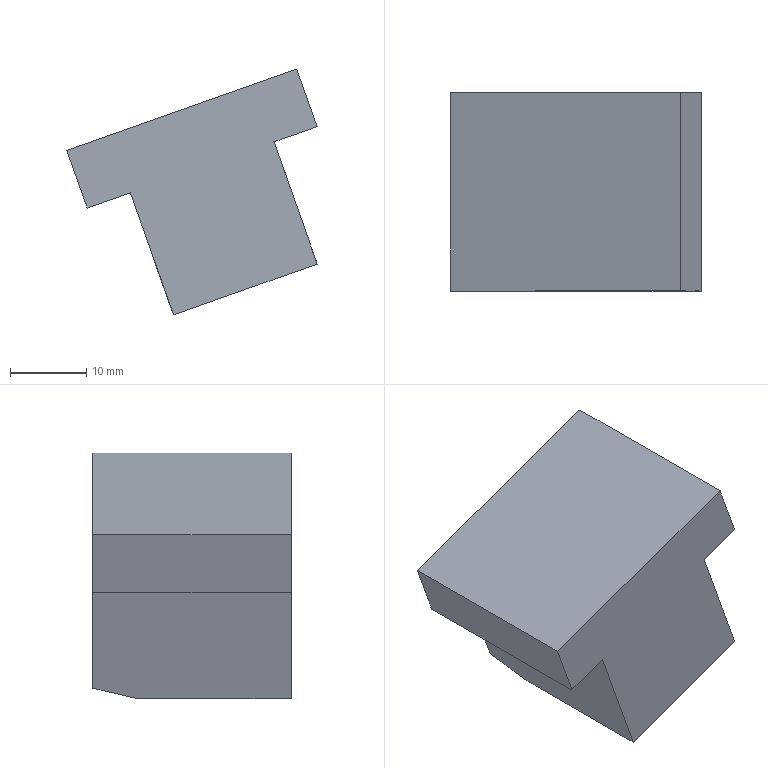Part | STEP file | T-BLOCK1_id174_x_t | 1 solid | 11 faces | box 32.854 x 26 x 32.245 mm | volume 15406 mm3 | plane 11
STEP:
#1=CARTESIAN_POINT('',(48.232,-40.,-222.441));
#2=VERTEX_POINT('',#1);
#3=CARTESIAN_POINT('',(67.085,-40.,-215.765));
#4=VERTEX_POINT('',#3);
#5=CARTESIAN_POINT('',(67.085,-40.,-215.765));
#6=DIRECTION('',(0.9426,0.,0.3338));
#7=VECTOR('',#6,1.);
#8=LINE('',#5,#7);
#9=EDGE_CURVE('',#2,#4,#8,.T.);
#10=ORIENTED_EDGE('',*,*,#9,.F.);
#11=CARTESIAN_POINT('',(47.733,-34.,-221.031));
#12=VERTEX_POINT('',#11);
#13=CARTESIAN_POINT('',(47.733,-34.,-221.031));
#14=DIRECTION('',(0.08076,-0.9703,-0.228));
#15=VECTOR('',#14,1.);
#16=LINE('',#13,#15);
#17=EDGE_CURVE('',#12,#2,#16,.T.);
#18=ORIENTED_EDGE('',*,*,#17,.F.);
#19=CARTESIAN_POINT('',(66.586,-34.,-214.355));
#20=VERTEX_POINT('',#19);
#21=CARTESIAN_POINT('',(66.586,-34.,-214.355));
#22=DIRECTION('',(-0.9426,0.,-0.3338));
#23=VECTOR('',#22,1.);
#24=LINE('',#21,#23);
#25=EDGE_CURVE('',#20,#12,#24,.T.);
#26=ORIENTED_EDGE('',*,*,#25,.F.);
#27=CARTESIAN_POINT('',(67.085,-40.,-215.765));
#28=DIRECTION('',(-0.08076,0.9703,0.228));
#29=VECTOR('',#28,1.);
#30=LINE('',#27,#29);
#31=EDGE_CURVE('',#4,#20,#30,.T.);
#32=ORIENTED_EDGE('',*,*,#31,.F.);
#33=EDGE_LOOP('',(#10,#18,#26,#32));
#34=FACE_OUTER_BOUND('',#33,.T.);
#35=CARTESIAN_POINT('',(1.1,-40.,-239.131));
#36=DIRECTION('',(-0.3239,-0.2419,0.9146));
#37=DIRECTION('',(0.9426,0.,0.3338));
#38=AXIS2_PLACEMENT_3D('',#35,#36,#37);
#39=PLANE('',#38);
#40=ADVANCED_FACE('',(#34),#39,.F.);
#41=CARTESIAN_POINT('',(48.232,-60.,-222.441));
#42=VERTEX_POINT('',#41);
#43=CARTESIAN_POINT('',(48.232,-60.,-222.441));
#44=DIRECTION('',(0.,-1.,0.));
#45=VECTOR('',#44,1.);
#46=LINE('',#43,#45);
#47=EDGE_CURVE('',#2,#42,#46,.T.);
#48=ORIENTED_EDGE('',*,*,#47,.F.);
#49=ORIENTED_EDGE('',*,*,#9,.T.);
#50=CARTESIAN_POINT('',(67.085,-60.,-215.765));
#51=VERTEX_POINT('',#50);
#52=CARTESIAN_POINT('',(67.085,-60.,-215.765));
#53=DIRECTION('',(0.,1.,0.));
#54=VECTOR('',#53,1.);
#55=LINE('',#52,#54);
#56=EDGE_CURVE('',#51,#4,#55,.T.);
#57=ORIENTED_EDGE('',*,*,#56,.F.);
#58=CARTESIAN_POINT('',(67.085,-60.,-215.765));
#59=DIRECTION('',(-0.9426,0.,-0.3338));
#60=VECTOR('',#59,1.);
#61=LINE('',#58,#60);
#62=EDGE_CURVE('',#51,#42,#61,.T.);
#63=ORIENTED_EDGE('',*,*,#62,.T.);
#64=EDGE_LOOP('',(#48,#49,#57,#63));
#65=FACE_OUTER_BOUND('',#64,.T.);
#66=CARTESIAN_POINT('',(67.085,-60.,-215.765));
#67=DIRECTION('',(0.3338,0.,-0.9426));
#68=DIRECTION('',(-0.9426,0.,-0.3338));
#69=AXIS2_PLACEMENT_3D('',#66,#67,#68);
#70=PLANE('',#69);
#71=ADVANCED_FACE('',(#65),#70,.T.);
#72=CARTESIAN_POINT('',(42.558,-34.,-206.416));
#73=VERTEX_POINT('',#72);
#74=CARTESIAN_POINT('',(47.733,-34.,-221.031));
#75=DIRECTION('',(-0.3338,0.,0.9426));
#76=VECTOR('',#75,1.);
#77=LINE('',#74,#76);
#78=EDGE_CURVE('',#12,#73,#77,.T.);
#79=ORIENTED_EDGE('',*,*,#78,.F.);
#80=ORIENTED_EDGE('',*,*,#17,.T.);
#81=ORIENTED_EDGE('',*,*,#47,.T.);
#82=CARTESIAN_POINT('',(42.558,-60.,-206.416));
#83=VERTEX_POINT('',#82);
#84=CARTESIAN_POINT('',(48.232,-60.,-222.441));
#85=DIRECTION('',(-0.3338,0.,0.9426));
#86=VECTOR('',#85,1.);
#87=LINE('',#84,#86);
#88=EDGE_CURVE('',#42,#83,#87,.T.);
#89=ORIENTED_EDGE('',*,*,#88,.T.);
#90=CARTESIAN_POINT('',(42.558,-60.,-206.416));
#91=DIRECTION('',(0.,-1.,0.));
#92=VECTOR('',#91,1.);
#93=LINE('',#90,#92);
#94=EDGE_CURVE('',#73,#83,#93,.T.);
#95=ORIENTED_EDGE('',*,*,#94,.F.);
#96=EDGE_LOOP('',(#79,#80,#81,#89,#95));
#97=FACE_OUTER_BOUND('',#96,.T.);
#98=CARTESIAN_POINT('',(48.232,-60.,-222.441));
#99=DIRECTION('',(-0.9426,0.,-0.3338));
#100=DIRECTION('',(-0.3338,0.,0.9426));
#101=AXIS2_PLACEMENT_3D('',#98,#99,#100);
#102=PLANE('',#101);
#103=ADVANCED_FACE('',(#97),#102,.T.);
#104=ORIENTED_EDGE('',*,*,#94,.T.);
#105=CARTESIAN_POINT('',(36.902,-60.,-208.419));
#106=VERTEX_POINT('',#105);
#107=CARTESIAN_POINT('',(42.558,-60.,-206.416));
#108=DIRECTION('',(-0.9426,0.,-0.3338));
#109=VECTOR('',#108,1.);
#110=LINE('',#107,#109);
#111=EDGE_CURVE('',#83,#106,#110,.T.);
#112=ORIENTED_EDGE('',*,*,#111,.T.);
#113=CARTESIAN_POINT('',(36.902,-34.,-208.419));
#114=VERTEX_POINT('',#113);
#115=CARTESIAN_POINT('',(36.902,-60.,-208.419));
#116=DIRECTION('',(0.,-1.,0.));
#117=VECTOR('',#116,1.);
#118=LINE('',#115,#117);
#119=EDGE_CURVE('',#114,#106,#118,.T.);
#120=ORIENTED_EDGE('',*,*,#119,.F.);
#121=CARTESIAN_POINT('',(42.558,-34.,-206.416));
#122=DIRECTION('',(-0.9426,0.,-0.3338));
#123=VECTOR('',#122,1.);
#124=LINE('',#121,#123);
#125=EDGE_CURVE('',#73,#114,#124,.T.);
#126=ORIENTED_EDGE('',*,*,#125,.F.);
#127=EDGE_LOOP('',(#104,#112,#120,#126));
#128=FACE_OUTER_BOUND('',#127,.T.);
#129=CARTESIAN_POINT('',(42.558,-60.,-206.416));
#130=DIRECTION('',(0.3338,0.,-0.9426));
#131=DIRECTION('',(-0.9426,0.,-0.3338));
#132=AXIS2_PLACEMENT_3D('',#129,#130,#131);
#133=PLANE('',#132);
#134=ADVANCED_FACE('',(#128),#133,.T.);
#135=CARTESIAN_POINT('',(67.066,-60.,-197.737));
#136=VERTEX_POINT('',#135);
#137=CARTESIAN_POINT('',(67.066,-34.,-197.737));
#138=VERTEX_POINT('',#137);
#139=CARTESIAN_POINT('',(67.066,-60.,-197.737));
#140=DIRECTION('',(0.,1.,0.));
#141=VECTOR('',#140,1.);
#142=LINE('',#139,#141);
#143=EDGE_CURVE('',#136,#138,#142,.T.);
#144=ORIENTED_EDGE('',*,*,#143,.F.);
#145=CARTESIAN_POINT('',(61.41,-60.,-199.74));
#146=VERTEX_POINT('',#145);
#147=CARTESIAN_POINT('',(67.066,-60.,-197.737));
#148=DIRECTION('',(-0.9426,0.,-0.3338));
#149=VECTOR('',#148,1.);
#150=LINE('',#147,#149);
#151=EDGE_CURVE('',#136,#146,#150,.T.);
#152=ORIENTED_EDGE('',*,*,#151,.T.);
#153=CARTESIAN_POINT('',(61.41,-34.,-199.74));
#154=VERTEX_POINT('',#153);
#155=CARTESIAN_POINT('',(61.41,-60.,-199.74));
#156=DIRECTION('',(0.,-1.,0.));
#157=VECTOR('',#156,1.);
#158=LINE('',#155,#157);
#159=EDGE_CURVE('',#154,#146,#158,.T.);
#160=ORIENTED_EDGE('',*,*,#159,.F.);
#161=CARTESIAN_POINT('',(67.066,-34.,-197.737));
#162=DIRECTION('',(-0.9426,0.,-0.3338));
#163=VECTOR('',#162,1.);
#164=LINE('',#161,#163);
#165=EDGE_CURVE('',#138,#154,#164,.T.);
#166=ORIENTED_EDGE('',*,*,#165,.F.);
#167=EDGE_LOOP('',(#144,#152,#160,#166));
#168=FACE_OUTER_BOUND('',#167,.T.);
#169=CARTESIAN_POINT('',(67.066,-60.,-197.737));
#170=DIRECTION('',(0.3338,0.,-0.9426));
#171=DIRECTION('',(-0.9426,0.,-0.3338));
#172=AXIS2_PLACEMENT_3D('',#169,#170,#171);
#173=PLANE('',#172);
#174=ADVANCED_FACE('',(#168),#173,.T.);
#175=ORIENTED_EDGE('',*,*,#56,.T.);
#176=ORIENTED_EDGE('',*,*,#31,.T.);
#177=CARTESIAN_POINT('',(61.41,-34.,-199.74));
#178=DIRECTION('',(0.3338,0.,-0.9426));
#179=VECTOR('',#178,1.);
#180=LINE('',#177,#179);
#181=EDGE_CURVE('',#154,#20,#180,.T.);
#182=ORIENTED_EDGE('',*,*,#181,.F.);
#183=ORIENTED_EDGE('',*,*,#159,.T.);
#184=CARTESIAN_POINT('',(61.41,-60.,-199.74));
#185=DIRECTION('',(0.3338,0.,-0.9426));
#186=VECTOR('',#185,1.);
#187=LINE('',#184,#186);
#188=EDGE_CURVE('',#146,#51,#187,.T.);
#189=ORIENTED_EDGE('',*,*,#188,.T.);
#190=EDGE_LOOP('',(#175,#176,#182,#183,#189));
#191=FACE_OUTER_BOUND('',#190,.T.);
#192=CARTESIAN_POINT('',(61.41,-60.,-199.74));
#193=DIRECTION('',(0.9426,0.,0.3338));
#194=DIRECTION('',(0.3338,0.,-0.9426));
#195=AXIS2_PLACEMENT_3D('',#192,#193,#194);
#196=PLANE('',#195);
#197=ADVANCED_FACE('',(#191),#196,.T.);
#198=CARTESIAN_POINT('',(64.396,-60.,-190.196));
#199=VERTEX_POINT('',#198);
#200=CARTESIAN_POINT('',(64.396,-34.,-190.196));
#201=VERTEX_POINT('',#200);
#202=CARTESIAN_POINT('',(64.396,-60.,-190.196));
#203=DIRECTION('',(0.,1.,0.));
#204=VECTOR('',#203,1.);
#205=LINE('',#202,#204);
#206=EDGE_CURVE('',#199,#201,#205,.T.);
#207=ORIENTED_EDGE('',*,*,#206,.F.);
#208=CARTESIAN_POINT('',(64.396,-60.,-190.196));
#209=DIRECTION('',(0.3338,0.,-0.9426));
#210=VECTOR('',#209,1.);
#211=LINE('',#208,#210);
#212=EDGE_CURVE('',#199,#136,#211,.T.);
#213=ORIENTED_EDGE('',*,*,#212,.T.);
#214=ORIENTED_EDGE('',*,*,#143,.T.);
#215=CARTESIAN_POINT('',(64.396,-34.,-190.196));
#216=DIRECTION('',(0.3338,0.,-0.9426));
#217=VECTOR('',#216,1.);
#218=LINE('',#215,#217);
#219=EDGE_CURVE('',#201,#138,#218,.T.);
#220=ORIENTED_EDGE('',*,*,#219,.F.);
#221=EDGE_LOOP('',(#207,#213,#214,#220));
#222=FACE_OUTER_BOUND('',#221,.T.);
#223=CARTESIAN_POINT('',(64.396,-60.,-190.196));
#224=DIRECTION('',(0.9426,0.,0.3338));
#225=DIRECTION('',(0.3338,0.,-0.9426));
#226=AXIS2_PLACEMENT_3D('',#223,#224,#225);
#227=PLANE('',#226);
#228=ADVANCED_FACE('',(#222),#227,.T.);
#229=ORIENTED_EDGE('',*,*,#181,.T.);
#230=ORIENTED_EDGE('',*,*,#25,.T.);
#231=ORIENTED_EDGE('',*,*,#78,.T.);
#232=ORIENTED_EDGE('',*,*,#125,.T.);
#233=CARTESIAN_POINT('',(34.231,-34.,-200.878));
#234=VERTEX_POINT('',#233);
#235=CARTESIAN_POINT('',(36.902,-34.,-208.419));
#236=DIRECTION('',(0.3338,0.,-0.9426));
#237=VECTOR('',#236,1.);
#238=LINE('',#235,#237);
#239=EDGE_CURVE('',#234,#114,#238,.T.);
#240=ORIENTED_EDGE('',*,*,#239,.F.);
#241=CARTESIAN_POINT('',(34.231,-34.,-200.878));
#242=DIRECTION('',(-0.9426,0.,-0.3338));
#243=VECTOR('',#242,1.);
#244=LINE('',#241,#243);
#245=EDGE_CURVE('',#201,#234,#244,.T.);
#246=ORIENTED_EDGE('',*,*,#245,.F.);
#247=ORIENTED_EDGE('',*,*,#219,.T.);
#248=ORIENTED_EDGE('',*,*,#165,.T.);
#249=EDGE_LOOP('',(#229,#230,#231,#232,#240,#246,#247,#248));
#250=FACE_OUTER_BOUND('',#249,.T.);
#251=CARTESIAN_POINT('',(1.1,-34.,-239.131));
#252=DIRECTION('',(0.,1.,0.));
#253=DIRECTION('',(0.,0.,1.));
#254=AXIS2_PLACEMENT_3D('',#251,#252,#253);
#255=PLANE('',#254);
#256=ADVANCED_FACE('',(#250),#255,.T.);
#257=ORIENTED_EDGE('',*,*,#119,.T.);
#258=CARTESIAN_POINT('',(34.231,-60.,-200.878));
#259=VERTEX_POINT('',#258);
#260=CARTESIAN_POINT('',(36.902,-60.,-208.419));
#261=DIRECTION('',(-0.3338,0.,0.9426));
#262=VECTOR('',#261,1.);
#263=LINE('',#260,#262);
#264=EDGE_CURVE('',#106,#259,#263,.T.);
#265=ORIENTED_EDGE('',*,*,#264,.T.);
#266=CARTESIAN_POINT('',(34.231,-60.,-200.878));
#267=DIRECTION('',(0.,-1.,0.));
#268=VECTOR('',#267,1.);
#269=LINE('',#266,#268);
#270=EDGE_CURVE('',#234,#259,#269,.T.);
#271=ORIENTED_EDGE('',*,*,#270,.F.);
#272=ORIENTED_EDGE('',*,*,#239,.T.);
#273=EDGE_LOOP('',(#257,#265,#271,#272));
#274=FACE_OUTER_BOUND('',#273,.T.);
#275=CARTESIAN_POINT('',(36.902,-60.,-208.419));
#276=DIRECTION('',(-0.9426,0.,-0.3338));
#277=DIRECTION('',(-0.3338,0.,0.9426));
#278=AXIS2_PLACEMENT_3D('',#275,#276,#277);
#279=PLANE('',#278);
#280=ADVANCED_FACE('',(#274),#279,.T.);
#281=ORIENTED_EDGE('',*,*,#151,.F.);
#282=ORIENTED_EDGE('',*,*,#212,.F.);
#283=CARTESIAN_POINT('',(34.231,-60.,-200.878));
#284=DIRECTION('',(0.9426,0.,0.3338));
#285=VECTOR('',#284,1.);
#286=LINE('',#283,#285);
#287=EDGE_CURVE('',#259,#199,#286,.T.);
#288=ORIENTED_EDGE('',*,*,#287,.F.);
#289=ORIENTED_EDGE('',*,*,#264,.F.);
#290=ORIENTED_EDGE('',*,*,#111,.F.);
#291=ORIENTED_EDGE('',*,*,#88,.F.);
#292=ORIENTED_EDGE('',*,*,#62,.F.);
#293=ORIENTED_EDGE('',*,*,#188,.F.);
#294=EDGE_LOOP('',(#281,#282,#288,#289,#290,#291,#292,#293));
#295=FACE_OUTER_BOUND('',#294,.T.);
#296=CARTESIAN_POINT('',(1.1,-60.,-239.131));
#297=DIRECTION('',(0.,1.,0.));
#298=DIRECTION('',(0.,0.,1.));
#299=AXIS2_PLACEMENT_3D('',#296,#297,#298);
#300=PLANE('',#299);
#301=ADVANCED_FACE('',(#295),#300,.F.);
#302=ORIENTED_EDGE('',*,*,#270,.T.);
#303=ORIENTED_EDGE('',*,*,#287,.T.);
#304=ORIENTED_EDGE('',*,*,#206,.T.);
#305=ORIENTED_EDGE('',*,*,#245,.T.);
#306=EDGE_LOOP('',(#302,#303,#304,#305));
#307=FACE_OUTER_BOUND('',#306,.T.);
#308=CARTESIAN_POINT('',(34.231,-60.,-200.878));
#309=DIRECTION('',(-0.3338,0.,0.9426));
#310=DIRECTION('',(0.9426,0.,0.3338));
#311=AXIS2_PLACEMENT_3D('',#308,#309,#310);
#312=PLANE('',#311);
#313=ADVANCED_FACE('',(#307),#312,.T.);
#314=CLOSED_SHELL('',(#40,#71,#103,#134,#174,#197,#228,#256,#280,#301,#313));
#315=MANIFOLD_SOLID_BREP('',#314);
#316=(LENGTH_UNIT()NAMED_UNIT(*)SI_UNIT(.MILLI.,.METRE.));
#317=UNCERTAINTY_MEASURE_WITH_UNIT(LENGTH_MEASURE(0.00002),#316,'','');
#318=(NAMED_UNIT(*)PLANE_ANGLE_UNIT()SI_UNIT($,.RADIAN.));
#319=PLANE_ANGLE_MEASURE_WITH_UNIT(PLANE_ANGLE_MEASURE(0.01745),#318);
#320=DIMENSIONAL_EXPONENTS(0.,0.,0.,0.,0.,0.,0.);
#321=(CONVERSION_BASED_UNIT('DEGREE',#319)NAMED_UNIT(#320)PLANE_ANGLE_UNIT());
#322=(NAMED_UNIT(*)SI_UNIT($,.STERADIAN.)SOLID_ANGLE_UNIT());
#323=(GEOMETRIC_REPRESENTATION_CONTEXT(3)GLOBAL_UNCERTAINTY_ASSIGNED_CONTEXT((#317))GLOBAL_UNIT_ASSIGNED_CONTEXT((#316,#321,#322))REPRESENTATION_CONTEXT('',''));
#324=ADVANCED_BREP_SHAPE_REPRESENTATION('',(#315),#323);